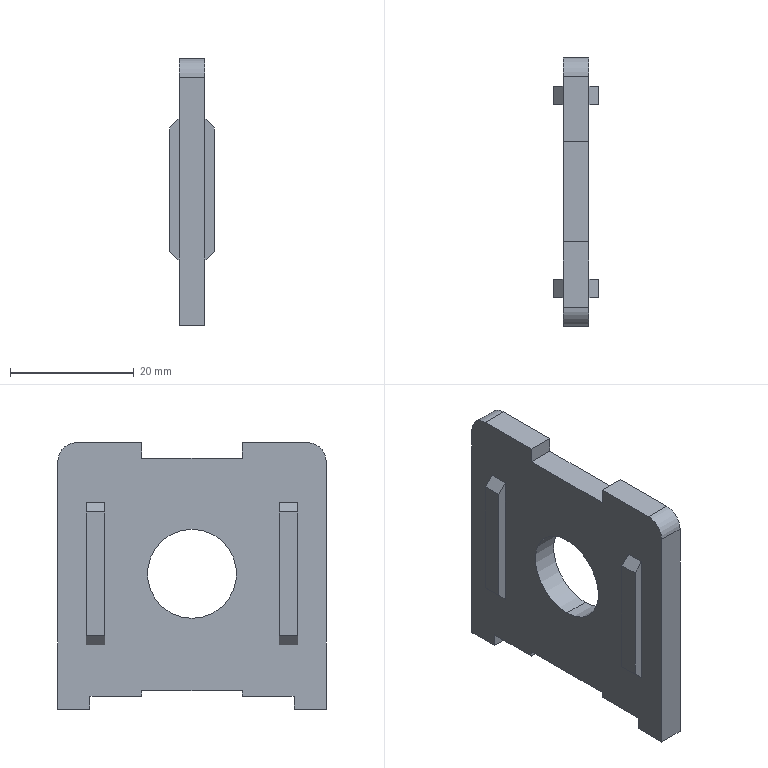Part | STEP file | _Y300T-A_SCREW | 1 solid | 42 faces | box 7.2 x 43.4 x 43.1 mm | volume 7021 mm3 | plane 38 | cylinder 4 | commonest cylinder face diameters 6 x2 14.4 x2
STEP:
#1=CARTESIAN_POINT('',(-2.1,0.,-7.2));
#2=VERTEX_POINT('',#1);
#3=CARTESIAN_POINT('',(-2.1,0.,7.2));
#4=VERTEX_POINT('',#3);
#5=CARTESIAN_POINT('',(-2.1,0.,0.));
#6=DIRECTION('',(-1.,0.,0.));
#7=DIRECTION('',(0.,0.,-1.));
#8=AXIS2_PLACEMENT_3D('',#5,#6,#7);
#9=CIRCLE('',#8,7.2);
#10=EDGE_CURVE('',#2,#4,#9,.T.);
#11=ORIENTED_EDGE('',*,*,#10,.T.);
#12=CARTESIAN_POINT('',(2.1,0.,7.2));
#13=VERTEX_POINT('',#12);
#14=CARTESIAN_POINT('',(2.1,0.,7.2));
#15=DIRECTION('',(1.,0.,0.));
#16=VECTOR('',#15,1000.);
#17=LINE('',#14,#16);
#18=EDGE_CURVE('',#4,#13,#17,.T.);
#19=ORIENTED_EDGE('',*,*,#18,.T.);
#20=CARTESIAN_POINT('',(2.1,0.,-7.2));
#21=VERTEX_POINT('',#20);
#22=CARTESIAN_POINT('',(2.1,0.,0.));
#23=DIRECTION('',(-1.,0.,0.));
#24=DIRECTION('',(0.,0.,-1.));
#25=AXIS2_PLACEMENT_3D('',#22,#23,#24);
#26=CIRCLE('',#25,7.2);
#27=EDGE_CURVE('',#21,#13,#26,.T.);
#28=ORIENTED_EDGE('',*,*,#27,.F.);
#29=CARTESIAN_POINT('',(2.1,0.,-7.2));
#30=DIRECTION('',(1.,0.,0.));
#31=VECTOR('',#30,1000.);
#32=LINE('',#29,#31);
#33=EDGE_CURVE('',#2,#21,#32,.T.);
#34=ORIENTED_EDGE('',*,*,#33,.F.);
#35=EDGE_LOOP('',(#11,#19,#28,#34));
#36=FACE_OUTER_BOUND('',#35,.T.);
#37=CARTESIAN_POINT('',(2.1,0.,0.));
#38=DIRECTION('',(1.,0.,0.));
#39=DIRECTION('',(0.,0.,-1.));
#40=AXIS2_PLACEMENT_3D('',#37,#38,#39);
#41=CYLINDRICAL_SURFACE('',#40,7.2);
#42=ADVANCED_FACE('',(#36),#41,.F.);
#43=CARTESIAN_POINT('',(-2.1,-14.1,-11.5));
#44=VERTEX_POINT('',#43);
#45=CARTESIAN_POINT('',(-2.1,-17.1,-11.5));
#46=VERTEX_POINT('',#45);
#47=CARTESIAN_POINT('',(-2.1,0.,-11.5));
#48=DIRECTION('',(0.,-1.,0.));
#49=VECTOR('',#48,1000.);
#50=LINE('',#47,#49);
#51=EDGE_CURVE('',#44,#46,#50,.T.);
#52=ORIENTED_EDGE('',*,*,#51,.F.);
#53=CARTESIAN_POINT('',(-2.1,-14.1,11.5));
#54=VERTEX_POINT('',#53);
#55=CARTESIAN_POINT('',(-2.1,-14.1,0.));
#56=DIRECTION('',(0.,0.,-1.));
#57=VECTOR('',#56,1000.);
#58=LINE('',#55,#57);
#59=EDGE_CURVE('',#54,#44,#58,.T.);
#60=ORIENTED_EDGE('',*,*,#59,.F.);
#61=CARTESIAN_POINT('',(-2.1,-17.1,11.5));
#62=VERTEX_POINT('',#61);
#63=CARTESIAN_POINT('',(-2.1,0.,11.5));
#64=DIRECTION('',(0.,1.,0.));
#65=VECTOR('',#64,1000.);
#66=LINE('',#63,#65);
#67=EDGE_CURVE('',#62,#54,#66,.T.);
#68=ORIENTED_EDGE('',*,*,#67,.F.);
#69=CARTESIAN_POINT('',(-2.1,-17.1,0.));
#70=DIRECTION('',(0.,0.,1.));
#71=VECTOR('',#70,1000.);
#72=LINE('',#69,#71);
#73=EDGE_CURVE('',#46,#62,#72,.T.);
#74=ORIENTED_EDGE('',*,*,#73,.F.);
#75=EDGE_LOOP('',(#52,#60,#68,#74));
#76=FACE_BOUND('',#75,.T.);
#77=CARTESIAN_POINT('',(-2.1,14.1,11.5));
#78=VERTEX_POINT('',#77);
#79=CARTESIAN_POINT('',(-2.1,17.1,11.5));
#80=VERTEX_POINT('',#79);
#81=CARTESIAN_POINT('',(-2.1,0.,11.5));
#82=DIRECTION('',(0.,1.,0.));
#83=VECTOR('',#82,1000.);
#84=LINE('',#81,#83);
#85=EDGE_CURVE('',#78,#80,#84,.T.);
#86=ORIENTED_EDGE('',*,*,#85,.F.);
#87=CARTESIAN_POINT('',(-2.1,14.1,-11.5));
#88=VERTEX_POINT('',#87);
#89=CARTESIAN_POINT('',(-2.1,14.1,0.));
#90=DIRECTION('',(0.,0.,1.));
#91=VECTOR('',#90,1000.);
#92=LINE('',#89,#91);
#93=EDGE_CURVE('',#88,#78,#92,.T.);
#94=ORIENTED_EDGE('',*,*,#93,.F.);
#95=CARTESIAN_POINT('',(-2.1,17.1,-11.5));
#96=VERTEX_POINT('',#95);
#97=CARTESIAN_POINT('',(-2.1,0.,-11.5));
#98=DIRECTION('',(0.,-1.,0.));
#99=VECTOR('',#98,1000.);
#100=LINE('',#97,#99);
#101=EDGE_CURVE('',#96,#88,#100,.T.);
#102=ORIENTED_EDGE('',*,*,#101,.F.);
#103=CARTESIAN_POINT('',(-2.1,17.1,0.));
#104=DIRECTION('',(0.,0.,-1.));
#105=VECTOR('',#104,1000.);
#106=LINE('',#103,#105);
#107=EDGE_CURVE('',#80,#96,#106,.T.);
#108=ORIENTED_EDGE('',*,*,#107,.F.);
#109=EDGE_LOOP('',(#86,#94,#102,#108));
#110=FACE_BOUND('',#109,.T.);
#111=ORIENTED_EDGE('',*,*,#10,.F.);
#112=CARTESIAN_POINT('',(-2.1,0.,0.));
#113=DIRECTION('',(-1.,0.,0.));
#114=DIRECTION('',(0.,0.,-1.));
#115=AXIS2_PLACEMENT_3D('',#112,#113,#114);
#116=CIRCLE('',#115,7.2);
#117=EDGE_CURVE('',#4,#2,#116,.T.);
#118=ORIENTED_EDGE('',*,*,#117,.F.);
#119=EDGE_LOOP('',(#111,#118));
#120=FACE_BOUND('',#119,.T.);
#121=CARTESIAN_POINT('',(-2.1,-16.5,-21.9));
#122=VERTEX_POINT('',#121);
#123=CARTESIAN_POINT('',(-2.1,-16.5,-19.8));
#124=VERTEX_POINT('',#123);
#125=CARTESIAN_POINT('',(-2.1,-16.5,0.));
#126=DIRECTION('',(0.,0.,1.));
#127=VECTOR('',#126,1000.);
#128=LINE('',#125,#127);
#129=EDGE_CURVE('',#122,#124,#128,.T.);
#130=ORIENTED_EDGE('',*,*,#129,.F.);
#131=CARTESIAN_POINT('',(-2.1,-21.7,-21.9));
#132=VERTEX_POINT('',#131);
#133=CARTESIAN_POINT('',(-2.1,0.,-21.9));
#134=DIRECTION('',(0.,1.,0.));
#135=VECTOR('',#134,1000.);
#136=LINE('',#133,#135);
#137=EDGE_CURVE('',#132,#122,#136,.T.);
#138=ORIENTED_EDGE('',*,*,#137,.F.);
#139=CARTESIAN_POINT('',(-2.1,-21.7,18.2));
#140=VERTEX_POINT('',#139);
#141=CARTESIAN_POINT('',(-2.1,-21.7,0.));
#142=DIRECTION('',(0.,0.,-1.));
#143=VECTOR('',#142,1000.);
#144=LINE('',#141,#143);
#145=EDGE_CURVE('',#140,#132,#144,.T.);
#146=ORIENTED_EDGE('',*,*,#145,.F.);
#147=CARTESIAN_POINT('',(-2.1,-18.7,21.2));
#148=VERTEX_POINT('',#147);
#149=CARTESIAN_POINT('',(-2.1,-18.7,18.2));
#150=DIRECTION('',(1.,0.,0.));
#151=DIRECTION('',(0.,0.,-1.));
#152=AXIS2_PLACEMENT_3D('',#149,#150,#151);
#153=CIRCLE('',#152,3.);
#154=EDGE_CURVE('',#148,#140,#153,.T.);
#155=ORIENTED_EDGE('',*,*,#154,.F.);
#156=CARTESIAN_POINT('',(-2.1,-8.1,21.2));
#157=VERTEX_POINT('',#156);
#158=CARTESIAN_POINT('',(-2.1,0.,21.2));
#159=DIRECTION('',(0.,-1.,0.));
#160=VECTOR('',#159,1000.);
#161=LINE('',#158,#160);
#162=EDGE_CURVE('',#157,#148,#161,.T.);
#163=ORIENTED_EDGE('',*,*,#162,.F.);
#164=CARTESIAN_POINT('',(-2.1,-8.1,18.7));
#165=VERTEX_POINT('',#164);
#166=CARTESIAN_POINT('',(-2.1,-8.1,0.));
#167=DIRECTION('',(0.,0.,1.));
#168=VECTOR('',#167,1000.);
#169=LINE('',#166,#168);
#170=EDGE_CURVE('',#165,#157,#169,.T.);
#171=ORIENTED_EDGE('',*,*,#170,.F.);
#172=CARTESIAN_POINT('',(-2.1,8.1,18.7));
#173=VERTEX_POINT('',#172);
#174=CARTESIAN_POINT('',(-2.1,0.,18.7));
#175=DIRECTION('',(0.,-1.,0.));
#176=VECTOR('',#175,1000.);
#177=LINE('',#174,#176);
#178=EDGE_CURVE('',#173,#165,#177,.T.);
#179=ORIENTED_EDGE('',*,*,#178,.F.);
#180=CARTESIAN_POINT('',(-2.1,8.1,21.2));
#181=VERTEX_POINT('',#180);
#182=CARTESIAN_POINT('',(-2.1,8.1,0.));
#183=DIRECTION('',(0.,0.,-1.));
#184=VECTOR('',#183,1000.);
#185=LINE('',#182,#184);
#186=EDGE_CURVE('',#181,#173,#185,.T.);
#187=ORIENTED_EDGE('',*,*,#186,.F.);
#188=CARTESIAN_POINT('',(-2.1,18.7,21.2));
#189=VERTEX_POINT('',#188);
#190=CARTESIAN_POINT('',(-2.1,0.,21.2));
#191=DIRECTION('',(0.,-1.,0.));
#192=VECTOR('',#191,1000.);
#193=LINE('',#190,#192);
#194=EDGE_CURVE('',#189,#181,#193,.T.);
#195=ORIENTED_EDGE('',*,*,#194,.F.);
#196=CARTESIAN_POINT('',(-2.1,21.7,18.2));
#197=VERTEX_POINT('',#196);
#198=CARTESIAN_POINT('',(-2.1,18.7,18.2));
#199=DIRECTION('',(1.,0.,0.));
#200=DIRECTION('',(0.,0.,-1.));
#201=AXIS2_PLACEMENT_3D('',#198,#199,#200);
#202=CIRCLE('',#201,3.);
#203=EDGE_CURVE('',#197,#189,#202,.T.);
#204=ORIENTED_EDGE('',*,*,#203,.F.);
#205=CARTESIAN_POINT('',(-2.1,21.7,-21.9));
#206=VERTEX_POINT('',#205);
#207=CARTESIAN_POINT('',(-2.1,21.7,0.));
#208=DIRECTION('',(0.,0.,1.));
#209=VECTOR('',#208,1000.);
#210=LINE('',#207,#209);
#211=EDGE_CURVE('',#206,#197,#210,.T.);
#212=ORIENTED_EDGE('',*,*,#211,.F.);
#213=CARTESIAN_POINT('',(-2.1,16.5,-21.9));
#214=VERTEX_POINT('',#213);
#215=CARTESIAN_POINT('',(-2.1,0.,-21.9));
#216=DIRECTION('',(0.,1.,0.));
#217=VECTOR('',#216,1000.);
#218=LINE('',#215,#217);
#219=EDGE_CURVE('',#214,#206,#218,.T.);
#220=ORIENTED_EDGE('',*,*,#219,.F.);
#221=CARTESIAN_POINT('',(-2.1,16.5,-19.8));
#222=VERTEX_POINT('',#221);
#223=CARTESIAN_POINT('',(-2.1,16.5,0.));
#224=DIRECTION('',(0.,0.,-1.));
#225=VECTOR('',#224,1000.);
#226=LINE('',#223,#225);
#227=EDGE_CURVE('',#222,#214,#226,.T.);
#228=ORIENTED_EDGE('',*,*,#227,.F.);
#229=CARTESIAN_POINT('',(-2.1,8.1,-19.8));
#230=VERTEX_POINT('',#229);
#231=CARTESIAN_POINT('',(-2.1,0.,-19.8));
#232=DIRECTION('',(0.,1.,0.));
#233=VECTOR('',#232,1000.);
#234=LINE('',#231,#233);
#235=EDGE_CURVE('',#230,#222,#234,.T.);
#236=ORIENTED_EDGE('',*,*,#235,.F.);
#237=CARTESIAN_POINT('',(-2.1,8.1,-18.9));
#238=VERTEX_POINT('',#237);
#239=CARTESIAN_POINT('',(-2.1,8.1,-18.9));
#240=DIRECTION('',(0.,0.,1.));
#241=VECTOR('',#240,1000.);
#242=LINE('',#239,#241);
#243=EDGE_CURVE('',#230,#238,#242,.T.);
#244=ORIENTED_EDGE('',*,*,#243,.T.);
#245=CARTESIAN_POINT('',(-2.1,-8.1,-18.9));
#246=VERTEX_POINT('',#245);
#247=CARTESIAN_POINT('',(-2.1,0.,-18.9));
#248=DIRECTION('',(0.,1.,0.));
#249=VECTOR('',#248,1000.);
#250=LINE('',#247,#249);
#251=EDGE_CURVE('',#246,#238,#250,.T.);
#252=ORIENTED_EDGE('',*,*,#251,.F.);
#253=CARTESIAN_POINT('',(-2.1,-8.1,-19.8));
#254=VERTEX_POINT('',#253);
#255=CARTESIAN_POINT('',(-2.1,-8.1,-21.9));
#256=DIRECTION('',(0.,0.,-1.));
#257=VECTOR('',#256,1000.);
#258=LINE('',#255,#257);
#259=EDGE_CURVE('',#246,#254,#258,.T.);
#260=ORIENTED_EDGE('',*,*,#259,.T.);
#261=CARTESIAN_POINT('',(-2.1,0.,-19.8));
#262=DIRECTION('',(0.,1.,0.));
#263=VECTOR('',#262,1000.);
#264=LINE('',#261,#263);
#265=EDGE_CURVE('',#124,#254,#264,.T.);
#266=ORIENTED_EDGE('',*,*,#265,.F.);
#267=EDGE_LOOP('',(#130,#138,#146,#155,#163,#171,#179,#187,#195,#204,#212,#220,#228,#236,#244,#252,#260,#266));
#268=FACE_OUTER_BOUND('',#267,.T.);
#269=CARTESIAN_POINT('',(-2.1,0.,0.));
#270=DIRECTION('',(1.,0.,0.));
#271=DIRECTION('',(0.,0.,-1.));
#272=AXIS2_PLACEMENT_3D('',#269,#270,#271);
#273=PLANE('',#272);
#274=ADVANCED_FACE('',(#76,#110,#120,#268),#273,.F.);
#275=CARTESIAN_POINT('',(-3.6,-17.1,-10.));
#276=VERTEX_POINT('',#275);
#277=CARTESIAN_POINT('',(-3.6,-17.1,10.));
#278=VERTEX_POINT('',#277);
#279=CARTESIAN_POINT('',(-3.6,-17.1,11.5));
#280=DIRECTION('',(0.,0.,1.));
#281=VECTOR('',#280,1000.);
#282=LINE('',#279,#281);
#283=EDGE_CURVE('',#276,#278,#282,.T.);
#284=ORIENTED_EDGE('',*,*,#283,.F.);
#285=CARTESIAN_POINT('',(-2.1,-17.1,-11.5));
#286=DIRECTION('',(-0.7071,0.,0.7071));
#287=VECTOR('',#286,1000.);
#288=LINE('',#285,#287);
#289=EDGE_CURVE('',#46,#276,#288,.T.);
#290=ORIENTED_EDGE('',*,*,#289,.F.);
#291=ORIENTED_EDGE('',*,*,#73,.T.);
#292=CARTESIAN_POINT('',(-3.6,-17.1,10.));
#293=DIRECTION('',(0.7071,0.,0.7071));
#294=VECTOR('',#293,1000.);
#295=LINE('',#292,#294);
#296=EDGE_CURVE('',#278,#62,#295,.T.);
#297=ORIENTED_EDGE('',*,*,#296,.F.);
#298=EDGE_LOOP('',(#284,#290,#291,#297));
#299=FACE_OUTER_BOUND('',#298,.T.);
#300=CARTESIAN_POINT('',(2.1,-17.1,11.5));
#301=DIRECTION('',(0.,1.,0.));
#302=DIRECTION('',(0.,0.,1.));
#303=AXIS2_PLACEMENT_3D('',#300,#301,#302);
#304=PLANE('',#303);
#305=ADVANCED_FACE('',(#299),#304,.F.);
#306=CARTESIAN_POINT('',(-3.6,-14.1,-10.));
#307=VERTEX_POINT('',#306);
#308=CARTESIAN_POINT('',(-2.1,-14.1,-11.5));
#309=DIRECTION('',(-0.7071,0.,0.7071));
#310=VECTOR('',#309,1000.);
#311=LINE('',#308,#310);
#312=EDGE_CURVE('',#44,#307,#311,.T.);
#313=ORIENTED_EDGE('',*,*,#312,.F.);
#314=ORIENTED_EDGE('',*,*,#51,.T.);
#315=ORIENTED_EDGE('',*,*,#289,.T.);
#316=CARTESIAN_POINT('',(-3.6,-14.1,-10.));
#317=DIRECTION('',(0.,-1.,0.));
#318=VECTOR('',#317,1000.);
#319=LINE('',#316,#318);
#320=EDGE_CURVE('',#307,#276,#319,.T.);
#321=ORIENTED_EDGE('',*,*,#320,.F.);
#322=EDGE_LOOP('',(#313,#314,#315,#321));
#323=FACE_OUTER_BOUND('',#322,.T.);
#324=CARTESIAN_POINT('',(-2.1,-14.1,-11.5));
#325=DIRECTION('',(0.7071,0.,0.7071));
#326=DIRECTION('',(0.7071,0.,-0.7071));
#327=AXIS2_PLACEMENT_3D('',#324,#325,#326);
#328=PLANE('',#327);
#329=ADVANCED_FACE('',(#323),#328,.F.);
#330=ORIENTED_EDGE('',*,*,#59,.T.);
#331=ORIENTED_EDGE('',*,*,#312,.T.);
#332=CARTESIAN_POINT('',(-3.6,-14.1,10.));
#333=VERTEX_POINT('',#332);
#334=CARTESIAN_POINT('',(-3.6,-14.1,0.));
#335=DIRECTION('',(0.,0.,1.));
#336=VECTOR('',#335,1000.);
#337=LINE('',#334,#336);
#338=EDGE_CURVE('',#307,#333,#337,.T.);
#339=ORIENTED_EDGE('',*,*,#338,.T.);
#340=CARTESIAN_POINT('',(-3.6,-14.1,10.));
#341=DIRECTION('',(0.7071,0.,0.7071));
#342=VECTOR('',#341,1000.);
#343=LINE('',#340,#342);
#344=EDGE_CURVE('',#333,#54,#343,.T.);
#345=ORIENTED_EDGE('',*,*,#344,.T.);
#346=EDGE_LOOP('',(#330,#331,#339,#345));
#347=FACE_OUTER_BOUND('',#346,.T.);
#348=CARTESIAN_POINT('',(0.,-14.1,0.));
#349=DIRECTION('',(0.,1.,0.));
#350=DIRECTION('',(0.,0.,1.));
#351=AXIS2_PLACEMENT_3D('',#348,#349,#350);
#352=PLANE('',#351);
#353=ADVANCED_FACE('',(#347),#352,.T.);
#354=ORIENTED_EDGE('',*,*,#344,.F.);
#355=CARTESIAN_POINT('',(-3.6,-14.1,10.));
#356=DIRECTION('',(0.,1.,0.));
#357=VECTOR('',#356,1000.);
#358=LINE('',#355,#357);
#359=EDGE_CURVE('',#278,#333,#358,.T.);
#360=ORIENTED_EDGE('',*,*,#359,.F.);
#361=ORIENTED_EDGE('',*,*,#296,.T.);
#362=ORIENTED_EDGE('',*,*,#67,.T.);
#363=EDGE_LOOP('',(#354,#360,#361,#362));
#364=FACE_OUTER_BOUND('',#363,.T.);
#365=CARTESIAN_POINT('',(-3.6,-14.1,10.));
#366=DIRECTION('',(0.7071,0.,-0.7071));
#367=DIRECTION('',(-0.7071,0.,-0.7071));
#368=AXIS2_PLACEMENT_3D('',#365,#366,#367);
#369=PLANE('',#368);
#370=ADVANCED_FACE('',(#364),#369,.F.);
#371=CARTESIAN_POINT('',(-3.6,17.1,10.));
#372=VERTEX_POINT('',#371);
#373=CARTESIAN_POINT('',(-3.6,17.1,-10.));
#374=VERTEX_POINT('',#373);
#375=CARTESIAN_POINT('',(-3.6,17.1,-21.9));
#376=DIRECTION('',(0.,0.,-1.));
#377=VECTOR('',#376,1000.);
#378=LINE('',#375,#377);
#379=EDGE_CURVE('',#372,#374,#378,.T.);
#380=ORIENTED_EDGE('',*,*,#379,.F.);
#381=CARTESIAN_POINT('',(-2.1,17.1,11.5));
#382=DIRECTION('',(-0.7071,0.,-0.7071));
#383=VECTOR('',#382,1000.);
#384=LINE('',#381,#383);
#385=EDGE_CURVE('',#80,#372,#384,.T.);
#386=ORIENTED_EDGE('',*,*,#385,.F.);
#387=ORIENTED_EDGE('',*,*,#107,.T.);
#388=CARTESIAN_POINT('',(-3.6,17.1,-10.));
#389=DIRECTION('',(0.7071,0.,-0.7071));
#390=VECTOR('',#389,1000.);
#391=LINE('',#388,#390);
#392=EDGE_CURVE('',#374,#96,#391,.T.);
#393=ORIENTED_EDGE('',*,*,#392,.F.);
#394=EDGE_LOOP('',(#380,#386,#387,#393));
#395=FACE_OUTER_BOUND('',#394,.T.);
#396=CARTESIAN_POINT('',(2.1,17.1,-21.9));
#397=DIRECTION('',(0.,-1.,0.));
#398=DIRECTION('',(0.,0.,-1.));
#399=AXIS2_PLACEMENT_3D('',#396,#397,#398);
#400=PLANE('',#399);
#401=ADVANCED_FACE('',(#395),#400,.F.);
#402=ORIENTED_EDGE('',*,*,#385,.T.);
#403=CARTESIAN_POINT('',(-3.6,14.1,10.));
#404=VERTEX_POINT('',#403);
#405=CARTESIAN_POINT('',(-3.6,14.1,10.));
#406=DIRECTION('',(0.,-1.,0.));
#407=VECTOR('',#406,1000.);
#408=LINE('',#405,#407);
#409=EDGE_CURVE('',#372,#404,#408,.T.);
#410=ORIENTED_EDGE('',*,*,#409,.T.);
#411=CARTESIAN_POINT('',(-3.6,14.1,10.));
#412=DIRECTION('',(0.7071,0.,0.7071));
#413=VECTOR('',#412,1000.);
#414=LINE('',#411,#413);
#415=EDGE_CURVE('',#404,#78,#414,.T.);
#416=ORIENTED_EDGE('',*,*,#415,.T.);
#417=ORIENTED_EDGE('',*,*,#85,.T.);
#418=EDGE_LOOP('',(#402,#410,#416,#417));
#419=FACE_OUTER_BOUND('',#418,.T.);
#420=CARTESIAN_POINT('',(-3.6,14.1,10.));
#421=DIRECTION('',(-0.7071,0.,0.7071));
#422=DIRECTION('',(0.7071,0.,0.7071));
#423=AXIS2_PLACEMENT_3D('',#420,#421,#422);
#424=PLANE('',#423);
#425=ADVANCED_FACE('',(#419),#424,.T.);
#426=ORIENTED_EDGE('',*,*,#415,.F.);
#427=CARTESIAN_POINT('',(-3.6,14.1,-10.));
#428=VERTEX_POINT('',#427);
#429=CARTESIAN_POINT('',(-3.6,14.1,0.));
#430=DIRECTION('',(0.,0.,1.));
#431=VECTOR('',#430,1000.);
#432=LINE('',#429,#431);
#433=EDGE_CURVE('',#428,#404,#432,.T.);
#434=ORIENTED_EDGE('',*,*,#433,.F.);
#435=CARTESIAN_POINT('',(-2.1,14.1,-11.5));
#436=DIRECTION('',(-0.7071,0.,0.7071));
#437=VECTOR('',#436,1000.);
#438=LINE('',#435,#437);
#439=EDGE_CURVE('',#88,#428,#438,.T.);
#440=ORIENTED_EDGE('',*,*,#439,.F.);
#441=ORIENTED_EDGE('',*,*,#93,.T.);
#442=EDGE_LOOP('',(#426,#434,#440,#441));
#443=FACE_OUTER_BOUND('',#442,.T.);
#444=CARTESIAN_POINT('',(0.,14.1,0.));
#445=DIRECTION('',(0.,1.,0.));
#446=DIRECTION('',(0.,0.,1.));
#447=AXIS2_PLACEMENT_3D('',#444,#445,#446);
#448=PLANE('',#447);
#449=ADVANCED_FACE('',(#443),#448,.F.);
#450=ORIENTED_EDGE('',*,*,#392,.T.);
#451=ORIENTED_EDGE('',*,*,#101,.T.);
#452=ORIENTED_EDGE('',*,*,#439,.T.);
#453=CARTESIAN_POINT('',(-3.6,14.1,-10.));
#454=DIRECTION('',(0.,1.,0.));
#455=VECTOR('',#454,1000.);
#456=LINE('',#453,#455);
#457=EDGE_CURVE('',#428,#374,#456,.T.);
#458=ORIENTED_EDGE('',*,*,#457,.T.);
#459=EDGE_LOOP('',(#450,#451,#452,#458));
#460=FACE_OUTER_BOUND('',#459,.T.);
#461=CARTESIAN_POINT('',(-2.1,14.1,-11.5));
#462=DIRECTION('',(-0.7071,0.,-0.7071));
#463=DIRECTION('',(-0.7071,0.,0.7071));
#464=AXIS2_PLACEMENT_3D('',#461,#462,#463);
#465=PLANE('',#464);
#466=ADVANCED_FACE('',(#460),#465,.T.);
#467=ORIENTED_EDGE('',*,*,#18,.F.);
#468=ORIENTED_EDGE('',*,*,#117,.T.);
#469=ORIENTED_EDGE('',*,*,#33,.T.);
#470=CARTESIAN_POINT('',(2.1,0.,0.));
#471=DIRECTION('',(-1.,0.,0.));
#472=DIRECTION('',(0.,0.,-1.));
#473=AXIS2_PLACEMENT_3D('',#470,#471,#472);
#474=CIRCLE('',#473,7.2);
#475=EDGE_CURVE('',#13,#21,#474,.T.);
#476=ORIENTED_EDGE('',*,*,#475,.F.);
#477=EDGE_LOOP('',(#467,#468,#469,#476));
#478=FACE_OUTER_BOUND('',#477,.T.);
#479=CARTESIAN_POINT('',(2.1,0.,0.));
#480=DIRECTION('',(1.,0.,0.));
#481=DIRECTION('',(0.,0.,-1.));
#482=AXIS2_PLACEMENT_3D('',#479,#480,#481);
#483=CYLINDRICAL_SURFACE('',#482,7.2);
#484=ADVANCED_FACE('',(#478),#483,.F.);
#485=CARTESIAN_POINT('',(2.1,-16.5,-19.8));
#486=VERTEX_POINT('',#485);
#487=CARTESIAN_POINT('',(2.1,-8.1,-19.8));
#488=VERTEX_POINT('',#487);
#489=CARTESIAN_POINT('',(2.1,-14.5,-19.8));
#490=DIRECTION('',(0.,1.,0.));
#491=VECTOR('',#490,1000.);
#492=LINE('',#489,#491);
#493=EDGE_CURVE('',#486,#488,#492,.T.);
#494=ORIENTED_EDGE('',*,*,#493,.F.);
#495=CARTESIAN_POINT('',(2.1,-16.5,-19.8));
#496=DIRECTION('',(1.,0.,0.));
#497=VECTOR('',#496,1000.);
#498=LINE('',#495,#497);
#499=EDGE_CURVE('',#124,#486,#498,.T.);
#500=ORIENTED_EDGE('',*,*,#499,.F.);
#501=ORIENTED_EDGE('',*,*,#265,.T.);
#502=CARTESIAN_POINT('',(2.1,-8.1,-19.8));
#503=DIRECTION('',(-1.,0.,0.));
#504=VECTOR('',#503,1000.);
#505=LINE('',#502,#504);
#506=EDGE_CURVE('',#488,#254,#505,.T.);
#507=ORIENTED_EDGE('',*,*,#506,.F.);
#508=EDGE_LOOP('',(#494,#500,#501,#507));
#509=FACE_OUTER_BOUND('',#508,.T.);
#510=CARTESIAN_POINT('',(2.1,-14.5,-19.8));
#511=DIRECTION('',(0.,0.,1.));
#512=DIRECTION('',(1.,0.,0.));
#513=AXIS2_PLACEMENT_3D('',#510,#511,#512);
#514=PLANE('',#513);
#515=ADVANCED_FACE('',(#509),#514,.F.);
#516=ORIENTED_EDGE('',*,*,#129,.T.);
#517=ORIENTED_EDGE('',*,*,#499,.T.);
#518=CARTESIAN_POINT('',(2.1,-16.5,-21.9));
#519=VERTEX_POINT('',#518);
#520=CARTESIAN_POINT('',(2.1,-16.5,-19.8));
#521=DIRECTION('',(0.,0.,-1.));
#522=VECTOR('',#521,1000.);
#523=LINE('',#520,#522);
#524=EDGE_CURVE('',#486,#519,#523,.T.);
#525=ORIENTED_EDGE('',*,*,#524,.T.);
#526=CARTESIAN_POINT('',(2.1,-16.5,-21.9));
#527=DIRECTION('',(-1.,0.,0.));
#528=VECTOR('',#527,1000.);
#529=LINE('',#526,#528);
#530=EDGE_CURVE('',#519,#122,#529,.T.);
#531=ORIENTED_EDGE('',*,*,#530,.T.);
#532=EDGE_LOOP('',(#516,#517,#525,#531));
#533=FACE_OUTER_BOUND('',#532,.T.);
#534=CARTESIAN_POINT('',(2.1,-16.5,-19.8));
#535=DIRECTION('',(0.,1.,0.));
#536=DIRECTION('',(0.,0.,1.));
#537=AXIS2_PLACEMENT_3D('',#534,#535,#536);
#538=PLANE('',#537);
#539=ADVANCED_FACE('',(#533),#538,.T.);
#540=CARTESIAN_POINT('',(2.1,-21.7,-21.9));
#541=VERTEX_POINT('',#540);
#542=CARTESIAN_POINT('',(2.1,-21.7,-21.9));
#543=DIRECTION('',(1.,0.,0.));
#544=VECTOR('',#543,1000.);
#545=LINE('',#542,#544);
#546=EDGE_CURVE('',#132,#541,#545,.T.);
#547=ORIENTED_EDGE('',*,*,#546,.F.);
#548=ORIENTED_EDGE('',*,*,#137,.T.);
#549=ORIENTED_EDGE('',*,*,#530,.F.);
#550=CARTESIAN_POINT('',(2.1,-17.1,-21.9));
#551=DIRECTION('',(0.,1.,0.));
#552=VECTOR('',#551,1000.);
#553=LINE('',#550,#552);
#554=EDGE_CURVE('',#541,#519,#553,.T.);
#555=ORIENTED_EDGE('',*,*,#554,.F.);
#556=EDGE_LOOP('',(#547,#548,#549,#555));
#557=FACE_OUTER_BOUND('',#556,.T.);
#558=CARTESIAN_POINT('',(2.1,-17.1,-21.9));
#559=DIRECTION('',(0.,0.,1.));
#560=DIRECTION('',(1.,0.,0.));
#561=AXIS2_PLACEMENT_3D('',#558,#559,#560);
#562=PLANE('',#561);
#563=ADVANCED_FACE('',(#557),#562,.F.);
#564=CARTESIAN_POINT('',(2.1,-21.7,18.2));
#565=VERTEX_POINT('',#564);
#566=CARTESIAN_POINT('',(2.1,-21.7,18.2));
#567=DIRECTION('',(0.,0.,-1.));
#568=VECTOR('',#567,1000.);
#569=LINE('',#566,#568);
#570=EDGE_CURVE('',#565,#541,#569,.T.);
#571=ORIENTED_EDGE('',*,*,#570,.F.);
#572=CARTESIAN_POINT('',(2.1,-21.7,18.2));
#573=DIRECTION('',(1.,0.,0.));
#574=VECTOR('',#573,1000.);
#575=LINE('',#572,#574);
#576=EDGE_CURVE('',#140,#565,#575,.T.);
#577=ORIENTED_EDGE('',*,*,#576,.F.);
#578=ORIENTED_EDGE('',*,*,#145,.T.);
#579=ORIENTED_EDGE('',*,*,#546,.T.);
#580=EDGE_LOOP('',(#571,#577,#578,#579));
#581=FACE_OUTER_BOUND('',#580,.T.);
#582=CARTESIAN_POINT('',(2.1,-21.7,18.2));
#583=DIRECTION('',(0.,1.,0.));
#584=DIRECTION('',(0.,0.,1.));
#585=AXIS2_PLACEMENT_3D('',#582,#583,#584);
#586=PLANE('',#585);
#587=ADVANCED_FACE('',(#581),#586,.F.);
#588=ORIENTED_EDGE('',*,*,#154,.T.);
#589=ORIENTED_EDGE('',*,*,#576,.T.);
#590=CARTESIAN_POINT('',(2.1,-18.7,21.2));
#591=VERTEX_POINT('',#590);
#592=CARTESIAN_POINT('',(2.1,-18.7,18.2));
#593=DIRECTION('',(-1.,0.,0.));
#594=DIRECTION('',(0.,0.,-1.));
#595=AXIS2_PLACEMENT_3D('',#592,#593,#594);
#596=CIRCLE('',#595,3.);
#597=EDGE_CURVE('',#565,#591,#596,.T.);
#598=ORIENTED_EDGE('',*,*,#597,.T.);
#599=CARTESIAN_POINT('',(2.1,-18.7,21.2));
#600=DIRECTION('',(-1.,0.,0.));
#601=VECTOR('',#600,1000.);
#602=LINE('',#599,#601);
#603=EDGE_CURVE('',#591,#148,#602,.T.);
#604=ORIENTED_EDGE('',*,*,#603,.T.);
#605=EDGE_LOOP('',(#588,#589,#598,#604));
#606=FACE_OUTER_BOUND('',#605,.T.);
#607=CARTESIAN_POINT('',(2.1,-18.7,18.2));
#608=DIRECTION('',(1.,0.,0.));
#609=DIRECTION('',(0.,0.,-1.));
#610=AXIS2_PLACEMENT_3D('',#607,#608,#609);
#611=CYLINDRICAL_SURFACE('',#610,3.);
#612=ADVANCED_FACE('',(#606),#611,.T.);
#613=CARTESIAN_POINT('',(2.1,-8.1,21.2));
#614=VERTEX_POINT('',#613);
#615=CARTESIAN_POINT('',(2.1,-8.1,21.2));
#616=DIRECTION('',(0.,-1.,0.));
#617=VECTOR('',#616,1000.);
#618=LINE('',#615,#617);
#619=EDGE_CURVE('',#614,#591,#618,.T.);
#620=ORIENTED_EDGE('',*,*,#619,.F.);
#621=CARTESIAN_POINT('',(2.1,-8.1,21.2));
#622=DIRECTION('',(1.,0.,0.));
#623=VECTOR('',#622,1000.);
#624=LINE('',#621,#623);
#625=EDGE_CURVE('',#157,#614,#624,.T.);
#626=ORIENTED_EDGE('',*,*,#625,.F.);
#627=ORIENTED_EDGE('',*,*,#162,.T.);
#628=ORIENTED_EDGE('',*,*,#603,.F.);
#629=EDGE_LOOP('',(#620,#626,#627,#628));
#630=FACE_OUTER_BOUND('',#629,.T.);
#631=CARTESIAN_POINT('',(2.1,-8.1,21.2));
#632=DIRECTION('',(0.,0.,-1.));
#633=DIRECTION('',(-1.,0.,0.));
#634=AXIS2_PLACEMENT_3D('',#631,#632,#633);
#635=PLANE('',#634);
#636=ADVANCED_FACE('',(#630),#635,.F.);
#637=CARTESIAN_POINT('',(2.1,-8.1,18.7));
#638=VERTEX_POINT('',#637);
#639=CARTESIAN_POINT('',(2.1,-8.1,18.7));
#640=DIRECTION('',(0.,0.,1.));
#641=VECTOR('',#640,1000.);
#642=LINE('',#639,#641);
#643=EDGE_CURVE('',#638,#614,#642,.T.);
#644=ORIENTED_EDGE('',*,*,#643,.F.);
#645=CARTESIAN_POINT('',(2.1,-8.1,18.7));
#646=DIRECTION('',(1.,0.,0.));
#647=VECTOR('',#646,1000.);
#648=LINE('',#645,#647);
#649=EDGE_CURVE('',#165,#638,#648,.T.);
#650=ORIENTED_EDGE('',*,*,#649,.F.);
#651=ORIENTED_EDGE('',*,*,#170,.T.);
#652=ORIENTED_EDGE('',*,*,#625,.T.);
#653=EDGE_LOOP('',(#644,#650,#651,#652));
#654=FACE_OUTER_BOUND('',#653,.T.);
#655=CARTESIAN_POINT('',(2.1,-8.1,18.7));
#656=DIRECTION('',(0.,-1.,0.));
#657=DIRECTION('',(0.,0.,-1.));
#658=AXIS2_PLACEMENT_3D('',#655,#656,#657);
#659=PLANE('',#658);
#660=ADVANCED_FACE('',(#654),#659,.F.);
#661=CARTESIAN_POINT('',(2.1,8.1,18.7));
#662=VERTEX_POINT('',#661);
#663=CARTESIAN_POINT('',(2.1,8.1,18.7));
#664=DIRECTION('',(0.,-1.,0.));
#665=VECTOR('',#664,1000.);
#666=LINE('',#663,#665);
#667=EDGE_CURVE('',#662,#638,#666,.T.);
#668=ORIENTED_EDGE('',*,*,#667,.F.);
#669=CARTESIAN_POINT('',(2.1,8.1,18.7));
#670=DIRECTION('',(1.,0.,0.));
#671=VECTOR('',#670,1000.);
#672=LINE('',#669,#671);
#673=EDGE_CURVE('',#173,#662,#672,.T.);
#674=ORIENTED_EDGE('',*,*,#673,.F.);
#675=ORIENTED_EDGE('',*,*,#178,.T.);
#676=ORIENTED_EDGE('',*,*,#649,.T.);
#677=EDGE_LOOP('',(#668,#674,#675,#676));
#678=FACE_OUTER_BOUND('',#677,.T.);
#679=CARTESIAN_POINT('',(2.1,8.1,18.7));
#680=DIRECTION('',(0.,0.,-1.));
#681=DIRECTION('',(-1.,0.,0.));
#682=AXIS2_PLACEMENT_3D('',#679,#680,#681);
#683=PLANE('',#682);
#684=ADVANCED_FACE('',(#678),#683,.F.);
#685=CARTESIAN_POINT('',(2.1,8.1,21.2));
#686=VERTEX_POINT('',#685);
#687=CARTESIAN_POINT('',(2.1,8.1,21.2));
#688=DIRECTION('',(0.,0.,-1.));
#689=VECTOR('',#688,1000.);
#690=LINE('',#687,#689);
#691=EDGE_CURVE('',#686,#662,#690,.T.);
#692=ORIENTED_EDGE('',*,*,#691,.F.);
#693=CARTESIAN_POINT('',(2.1,8.1,21.2));
#694=DIRECTION('',(1.,0.,0.));
#695=VECTOR('',#694,1000.);
#696=LINE('',#693,#695);
#697=EDGE_CURVE('',#181,#686,#696,.T.);
#698=ORIENTED_EDGE('',*,*,#697,.F.);
#699=ORIENTED_EDGE('',*,*,#186,.T.);
#700=ORIENTED_EDGE('',*,*,#673,.T.);
#701=EDGE_LOOP('',(#692,#698,#699,#700));
#702=FACE_OUTER_BOUND('',#701,.T.);
#703=CARTESIAN_POINT('',(2.1,8.1,21.2));
#704=DIRECTION('',(0.,1.,0.));
#705=DIRECTION('',(0.,0.,1.));
#706=AXIS2_PLACEMENT_3D('',#703,#704,#705);
#707=PLANE('',#706);
#708=ADVANCED_FACE('',(#702),#707,.F.);
#709=CARTESIAN_POINT('',(2.1,18.7,21.2));
#710=VERTEX_POINT('',#709);
#711=CARTESIAN_POINT('',(2.1,13.569,21.2));
#712=DIRECTION('',(0.,-1.,0.));
#713=VECTOR('',#712,1000.);
#714=LINE('',#711,#713);
#715=EDGE_CURVE('',#710,#686,#714,.T.);
#716=ORIENTED_EDGE('',*,*,#715,.F.);
#717=CARTESIAN_POINT('',(2.1,18.7,21.2));
#718=DIRECTION('',(1.,0.,0.));
#719=VECTOR('',#718,1000.);
#720=LINE('',#717,#719);
#721=EDGE_CURVE('',#189,#710,#720,.T.);
#722=ORIENTED_EDGE('',*,*,#721,.F.);
#723=ORIENTED_EDGE('',*,*,#194,.T.);
#724=ORIENTED_EDGE('',*,*,#697,.T.);
#725=EDGE_LOOP('',(#716,#722,#723,#724));
#726=FACE_OUTER_BOUND('',#725,.T.);
#727=CARTESIAN_POINT('',(2.1,13.569,21.2));
#728=DIRECTION('',(0.,0.,-1.));
#729=DIRECTION('',(-1.,0.,0.));
#730=AXIS2_PLACEMENT_3D('',#727,#728,#729);
#731=PLANE('',#730);
#732=ADVANCED_FACE('',(#726),#731,.F.);
#733=ORIENTED_EDGE('',*,*,#203,.T.);
#734=ORIENTED_EDGE('',*,*,#721,.T.);
#735=CARTESIAN_POINT('',(2.1,21.7,18.2));
#736=VERTEX_POINT('',#735);
#737=CARTESIAN_POINT('',(2.1,18.7,18.2));
#738=DIRECTION('',(-1.,0.,0.));
#739=DIRECTION('',(0.,0.,-1.));
#740=AXIS2_PLACEMENT_3D('',#737,#738,#739);
#741=CIRCLE('',#740,3.);
#742=EDGE_CURVE('',#710,#736,#741,.T.);
#743=ORIENTED_EDGE('',*,*,#742,.T.);
#744=CARTESIAN_POINT('',(2.1,21.7,18.2));
#745=DIRECTION('',(-1.,0.,0.));
#746=VECTOR('',#745,1000.);
#747=LINE('',#744,#746);
#748=EDGE_CURVE('',#736,#197,#747,.T.);
#749=ORIENTED_EDGE('',*,*,#748,.T.);
#750=EDGE_LOOP('',(#733,#734,#743,#749));
#751=FACE_OUTER_BOUND('',#750,.T.);
#752=CARTESIAN_POINT('',(2.1,18.7,18.2));
#753=DIRECTION('',(1.,0.,0.));
#754=DIRECTION('',(0.,0.,-1.));
#755=AXIS2_PLACEMENT_3D('',#752,#753,#754);
#756=CYLINDRICAL_SURFACE('',#755,3.);
#757=ADVANCED_FACE('',(#751),#756,.T.);
#758=CARTESIAN_POINT('',(2.1,21.7,-21.9));
#759=VERTEX_POINT('',#758);
#760=CARTESIAN_POINT('',(2.1,21.7,-21.9));
#761=DIRECTION('',(0.,0.,1.));
#762=VECTOR('',#761,1000.);
#763=LINE('',#760,#762);
#764=EDGE_CURVE('',#759,#736,#763,.T.);
#765=ORIENTED_EDGE('',*,*,#764,.F.);
#766=CARTESIAN_POINT('',(2.1,21.7,-21.9));
#767=DIRECTION('',(1.,0.,0.));
#768=VECTOR('',#767,1000.);
#769=LINE('',#766,#768);
#770=EDGE_CURVE('',#206,#759,#769,.T.);
#771=ORIENTED_EDGE('',*,*,#770,.F.);
#772=ORIENTED_EDGE('',*,*,#211,.T.);
#773=ORIENTED_EDGE('',*,*,#748,.F.);
#774=EDGE_LOOP('',(#765,#771,#772,#773));
#775=FACE_OUTER_BOUND('',#774,.T.);
#776=CARTESIAN_POINT('',(2.1,21.7,-21.9));
#777=DIRECTION('',(0.,-1.,0.));
#778=DIRECTION('',(0.,0.,-1.));
#779=AXIS2_PLACEMENT_3D('',#776,#777,#778);
#780=PLANE('',#779);
#781=ADVANCED_FACE('',(#775),#780,.F.);
#782=ORIENTED_EDGE('',*,*,#770,.T.);
#783=CARTESIAN_POINT('',(2.1,16.5,-21.9));
#784=VERTEX_POINT('',#783);
#785=CARTESIAN_POINT('',(2.1,14.5,-21.9));
#786=DIRECTION('',(0.,1.,0.));
#787=VECTOR('',#786,1000.);
#788=LINE('',#785,#787);
#789=EDGE_CURVE('',#784,#759,#788,.T.);
#790=ORIENTED_EDGE('',*,*,#789,.F.);
#791=CARTESIAN_POINT('',(2.1,16.5,-21.9));
#792=DIRECTION('',(1.,0.,0.));
#793=VECTOR('',#792,1000.);
#794=LINE('',#791,#793);
#795=EDGE_CURVE('',#214,#784,#794,.T.);
#796=ORIENTED_EDGE('',*,*,#795,.F.);
#797=ORIENTED_EDGE('',*,*,#219,.T.);
#798=EDGE_LOOP('',(#782,#790,#796,#797));
#799=FACE_OUTER_BOUND('',#798,.T.);
#800=CARTESIAN_POINT('',(2.1,14.5,-21.9));
#801=DIRECTION('',(0.,0.,1.));
#802=DIRECTION('',(1.,0.,0.));
#803=AXIS2_PLACEMENT_3D('',#800,#801,#802);
#804=PLANE('',#803);
#805=ADVANCED_FACE('',(#799),#804,.F.);
#806=ORIENTED_EDGE('',*,*,#227,.T.);
#807=ORIENTED_EDGE('',*,*,#795,.T.);
#808=CARTESIAN_POINT('',(2.1,16.5,-19.8));
#809=VERTEX_POINT('',#808);
#810=CARTESIAN_POINT('',(2.1,16.5,-21.9));
#811=DIRECTION('',(0.,0.,1.));
#812=VECTOR('',#811,1000.);
#813=LINE('',#810,#812);
#814=EDGE_CURVE('',#784,#809,#813,.T.);
#815=ORIENTED_EDGE('',*,*,#814,.T.);
#816=CARTESIAN_POINT('',(2.1,16.5,-19.8));
#817=DIRECTION('',(-1.,0.,0.));
#818=VECTOR('',#817,1000.);
#819=LINE('',#816,#818);
#820=EDGE_CURVE('',#809,#222,#819,.T.);
#821=ORIENTED_EDGE('',*,*,#820,.T.);
#822=EDGE_LOOP('',(#806,#807,#815,#821));
#823=FACE_OUTER_BOUND('',#822,.T.);
#824=CARTESIAN_POINT('',(2.1,16.5,-21.9));
#825=DIRECTION('',(0.,-1.,0.));
#826=DIRECTION('',(0.,0.,-1.));
#827=AXIS2_PLACEMENT_3D('',#824,#825,#826);
#828=PLANE('',#827);
#829=ADVANCED_FACE('',(#823),#828,.T.);
#830=CARTESIAN_POINT('',(2.1,8.1,-19.8));
#831=VERTEX_POINT('',#830);
#832=CARTESIAN_POINT('',(2.1,12.,-19.8));
#833=DIRECTION('',(0.,1.,0.));
#834=VECTOR('',#833,1000.);
#835=LINE('',#832,#834);
#836=EDGE_CURVE('',#831,#809,#835,.T.);
#837=ORIENTED_EDGE('',*,*,#836,.F.);
#838=CARTESIAN_POINT('',(2.1,8.1,-19.8));
#839=DIRECTION('',(1.,0.,0.));
#840=VECTOR('',#839,1000.);
#841=LINE('',#838,#840);
#842=EDGE_CURVE('',#230,#831,#841,.T.);
#843=ORIENTED_EDGE('',*,*,#842,.F.);
#844=ORIENTED_EDGE('',*,*,#235,.T.);
#845=ORIENTED_EDGE('',*,*,#820,.F.);
#846=EDGE_LOOP('',(#837,#843,#844,#845));
#847=FACE_OUTER_BOUND('',#846,.T.);
#848=CARTESIAN_POINT('',(2.1,12.,-19.8));
#849=DIRECTION('',(0.,0.,1.));
#850=DIRECTION('',(1.,0.,0.));
#851=AXIS2_PLACEMENT_3D('',#848,#849,#850);
#852=PLANE('',#851);
#853=ADVANCED_FACE('',(#847),#852,.F.);
#854=CARTESIAN_POINT('',(2.1,-8.1,-18.9));
#855=VERTEX_POINT('',#854);
#856=CARTESIAN_POINT('',(2.1,8.1,-18.9));
#857=VERTEX_POINT('',#856);
#858=CARTESIAN_POINT('',(2.1,-8.1,-18.9));
#859=DIRECTION('',(0.,1.,0.));
#860=VECTOR('',#859,1000.);
#861=LINE('',#858,#860);
#862=EDGE_CURVE('',#855,#857,#861,.T.);
#863=ORIENTED_EDGE('',*,*,#862,.F.);
#864=CARTESIAN_POINT('',(2.1,-8.1,-18.9));
#865=DIRECTION('',(1.,0.,0.));
#866=VECTOR('',#865,1000.);
#867=LINE('',#864,#866);
#868=EDGE_CURVE('',#246,#855,#867,.T.);
#869=ORIENTED_EDGE('',*,*,#868,.F.);
#870=ORIENTED_EDGE('',*,*,#251,.T.);
#871=CARTESIAN_POINT('',(2.1,8.1,-18.9));
#872=DIRECTION('',(-1.,0.,0.));
#873=VECTOR('',#872,1000.);
#874=LINE('',#871,#873);
#875=EDGE_CURVE('',#857,#238,#874,.T.);
#876=ORIENTED_EDGE('',*,*,#875,.F.);
#877=EDGE_LOOP('',(#863,#869,#870,#876));
#878=FACE_OUTER_BOUND('',#877,.T.);
#879=CARTESIAN_POINT('',(2.1,-8.1,-18.9));
#880=DIRECTION('',(0.,0.,1.));
#881=DIRECTION('',(1.,0.,0.));
#882=AXIS2_PLACEMENT_3D('',#879,#880,#881);
#883=PLANE('',#882);
#884=ADVANCED_FACE('',(#878),#883,.F.);
#885=ORIENTED_EDGE('',*,*,#338,.F.);
#886=ORIENTED_EDGE('',*,*,#320,.T.);
#887=ORIENTED_EDGE('',*,*,#283,.T.);
#888=ORIENTED_EDGE('',*,*,#359,.T.);
#889=EDGE_LOOP('',(#885,#886,#887,#888));
#890=FACE_OUTER_BOUND('',#889,.T.);
#891=CARTESIAN_POINT('',(-3.6,-14.1,-10.));
#892=DIRECTION('',(1.,0.,0.));
#893=DIRECTION('',(0.,0.,-1.));
#894=AXIS2_PLACEMENT_3D('',#891,#892,#893);
#895=PLANE('',#894);
#896=ADVANCED_FACE('',(#890),#895,.F.);
#897=ORIENTED_EDGE('',*,*,#379,.T.);
#898=ORIENTED_EDGE('',*,*,#457,.F.);
#899=ORIENTED_EDGE('',*,*,#433,.T.);
#900=ORIENTED_EDGE('',*,*,#409,.F.);
#901=EDGE_LOOP('',(#897,#898,#899,#900));
#902=FACE_OUTER_BOUND('',#901,.T.);
#903=CARTESIAN_POINT('',(-3.6,14.1,-10.));
#904=DIRECTION('',(-1.,0.,0.));
#905=DIRECTION('',(0.,0.,1.));
#906=AXIS2_PLACEMENT_3D('',#903,#904,#905);
#907=PLANE('',#906);
#908=ADVANCED_FACE('',(#902),#907,.T.);
#909=CARTESIAN_POINT('',(2.1,-17.1,-11.5));
#910=VERTEX_POINT('',#909);
#911=CARTESIAN_POINT('',(2.1,-17.1,11.5));
#912=VERTEX_POINT('',#911);
#913=CARTESIAN_POINT('',(2.1,-17.1,0.));
#914=DIRECTION('',(0.,0.,1.));
#915=VECTOR('',#914,1000.);
#916=LINE('',#913,#915);
#917=EDGE_CURVE('',#910,#912,#916,.T.);
#918=ORIENTED_EDGE('',*,*,#917,.T.);
#919=CARTESIAN_POINT('',(2.1,-14.1,11.5));
#920=VERTEX_POINT('',#919);
#921=CARTESIAN_POINT('',(2.1,0.,11.5));
#922=DIRECTION('',(0.,1.,0.));
#923=VECTOR('',#922,1000.);
#924=LINE('',#921,#923);
#925=EDGE_CURVE('',#912,#920,#924,.T.);
#926=ORIENTED_EDGE('',*,*,#925,.T.);
#927=CARTESIAN_POINT('',(2.1,-14.1,-11.5));
#928=VERTEX_POINT('',#927);
#929=CARTESIAN_POINT('',(2.1,-14.1,0.));
#930=DIRECTION('',(0.,0.,-1.));
#931=VECTOR('',#930,1000.);
#932=LINE('',#929,#931);
#933=EDGE_CURVE('',#920,#928,#932,.T.);
#934=ORIENTED_EDGE('',*,*,#933,.T.);
#935=CARTESIAN_POINT('',(2.1,0.,-11.5));
#936=DIRECTION('',(0.,-1.,0.));
#937=VECTOR('',#936,1000.);
#938=LINE('',#935,#937);
#939=EDGE_CURVE('',#928,#910,#938,.T.);
#940=ORIENTED_EDGE('',*,*,#939,.T.);
#941=EDGE_LOOP('',(#918,#926,#934,#940));
#942=FACE_BOUND('',#941,.T.);
#943=CARTESIAN_POINT('',(2.1,17.1,11.5));
#944=VERTEX_POINT('',#943);
#945=CARTESIAN_POINT('',(2.1,17.1,-11.5));
#946=VERTEX_POINT('',#945);
#947=CARTESIAN_POINT('',(2.1,17.1,0.));
#948=DIRECTION('',(0.,0.,-1.));
#949=VECTOR('',#948,1000.);
#950=LINE('',#947,#949);
#951=EDGE_CURVE('',#944,#946,#950,.T.);
#952=ORIENTED_EDGE('',*,*,#951,.T.);
#953=CARTESIAN_POINT('',(2.1,14.1,-11.5));
#954=VERTEX_POINT('',#953);
#955=CARTESIAN_POINT('',(2.1,0.,-11.5));
#956=DIRECTION('',(0.,-1.,0.));
#957=VECTOR('',#956,1000.);
#958=LINE('',#955,#957);
#959=EDGE_CURVE('',#946,#954,#958,.T.);
#960=ORIENTED_EDGE('',*,*,#959,.T.);
#961=CARTESIAN_POINT('',(2.1,14.1,11.5));
#962=VERTEX_POINT('',#961);
#963=CARTESIAN_POINT('',(2.1,14.1,0.));
#964=DIRECTION('',(0.,0.,1.));
#965=VECTOR('',#964,1000.);
#966=LINE('',#963,#965);
#967=EDGE_CURVE('',#954,#962,#966,.T.);
#968=ORIENTED_EDGE('',*,*,#967,.T.);
#969=CARTESIAN_POINT('',(2.1,0.,11.5));
#970=DIRECTION('',(0.,1.,0.));
#971=VECTOR('',#970,1000.);
#972=LINE('',#969,#971);
#973=EDGE_CURVE('',#962,#944,#972,.T.);
#974=ORIENTED_EDGE('',*,*,#973,.T.);
#975=EDGE_LOOP('',(#952,#960,#968,#974));
#976=FACE_BOUND('',#975,.T.);
#977=ORIENTED_EDGE('',*,*,#27,.T.);
#978=ORIENTED_EDGE('',*,*,#475,.T.);
#979=EDGE_LOOP('',(#977,#978));
#980=FACE_BOUND('',#979,.T.);
#981=ORIENTED_EDGE('',*,*,#597,.F.);
#982=ORIENTED_EDGE('',*,*,#570,.T.);
#983=ORIENTED_EDGE('',*,*,#554,.T.);
#984=ORIENTED_EDGE('',*,*,#524,.F.);
#985=ORIENTED_EDGE('',*,*,#493,.T.);
#986=CARTESIAN_POINT('',(2.1,-8.1,0.));
#987=DIRECTION('',(0.,0.,1.));
#988=VECTOR('',#987,1000.);
#989=LINE('',#986,#988);
#990=EDGE_CURVE('',#488,#855,#989,.T.);
#991=ORIENTED_EDGE('',*,*,#990,.T.);
#992=ORIENTED_EDGE('',*,*,#862,.T.);
#993=CARTESIAN_POINT('',(2.1,8.1,0.));
#994=DIRECTION('',(0.,0.,-1.));
#995=VECTOR('',#994,1000.);
#996=LINE('',#993,#995);
#997=EDGE_CURVE('',#857,#831,#996,.T.);
#998=ORIENTED_EDGE('',*,*,#997,.T.);
#999=ORIENTED_EDGE('',*,*,#836,.T.);
#1000=ORIENTED_EDGE('',*,*,#814,.F.);
#1001=ORIENTED_EDGE('',*,*,#789,.T.);
#1002=ORIENTED_EDGE('',*,*,#764,.T.);
#1003=ORIENTED_EDGE('',*,*,#742,.F.);
#1004=ORIENTED_EDGE('',*,*,#715,.T.);
#1005=ORIENTED_EDGE('',*,*,#691,.T.);
#1006=ORIENTED_EDGE('',*,*,#667,.T.);
#1007=ORIENTED_EDGE('',*,*,#643,.T.);
#1008=ORIENTED_EDGE('',*,*,#619,.T.);
#1009=EDGE_LOOP('',(#981,#982,#983,#984,#985,#991,#992,#998,#999,#1000,#1001,#1002,#1003,#1004,#1005,#1006,#1007,#1008));
#1010=FACE_OUTER_BOUND('',#1009,.T.);
#1011=CARTESIAN_POINT('',(2.1,0.,0.));
#1012=DIRECTION('',(1.,0.,0.));
#1013=DIRECTION('',(0.,0.,-1.));
#1014=AXIS2_PLACEMENT_3D('',#1011,#1012,#1013);
#1015=PLANE('',#1014);
#1016=ADVANCED_FACE('',(#942,#976,#980,#1010),#1015,.T.);
#1017=ORIENTED_EDGE('',*,*,#868,.T.);
#1018=ORIENTED_EDGE('',*,*,#990,.F.);
#1019=ORIENTED_EDGE('',*,*,#506,.T.);
#1020=ORIENTED_EDGE('',*,*,#259,.F.);
#1021=EDGE_LOOP('',(#1017,#1018,#1019,#1020));
#1022=FACE_OUTER_BOUND('',#1021,.T.);
#1023=CARTESIAN_POINT('',(2.1,-8.1,-21.9));
#1024=DIRECTION('',(0.,-1.,0.));
#1025=DIRECTION('',(0.,0.,-1.));
#1026=AXIS2_PLACEMENT_3D('',#1023,#1024,#1025);
#1027=PLANE('',#1026);
#1028=ADVANCED_FACE('',(#1022),#1027,.F.);
#1029=ORIENTED_EDGE('',*,*,#875,.T.);
#1030=ORIENTED_EDGE('',*,*,#243,.F.);
#1031=ORIENTED_EDGE('',*,*,#842,.T.);
#1032=ORIENTED_EDGE('',*,*,#997,.F.);
#1033=EDGE_LOOP('',(#1029,#1030,#1031,#1032));
#1034=FACE_OUTER_BOUND('',#1033,.T.);
#1035=CARTESIAN_POINT('',(2.1,8.1,-18.9));
#1036=DIRECTION('',(0.,1.,0.));
#1037=DIRECTION('',(0.,0.,1.));
#1038=AXIS2_PLACEMENT_3D('',#1035,#1036,#1037);
#1039=PLANE('',#1038);
#1040=ADVANCED_FACE('',(#1034),#1039,.F.);
#1041=CARTESIAN_POINT('',(3.6,-14.1,10.));
#1042=VERTEX_POINT('',#1041);
#1043=CARTESIAN_POINT('',(2.1,-14.1,11.5));
#1044=DIRECTION('',(0.7071,0.,-0.7071));
#1045=VECTOR('',#1044,1000.);
#1046=LINE('',#1043,#1045);
#1047=EDGE_CURVE('',#920,#1042,#1046,.T.);
#1048=ORIENTED_EDGE('',*,*,#1047,.F.);
#1049=ORIENTED_EDGE('',*,*,#925,.F.);
#1050=CARTESIAN_POINT('',(3.6,-17.1,10.));
#1051=VERTEX_POINT('',#1050);
#1052=CARTESIAN_POINT('',(2.1,-17.1,11.5));
#1053=DIRECTION('',(-0.7071,0.,0.7071));
#1054=VECTOR('',#1053,1000.);
#1055=LINE('',#1052,#1054);
#1056=EDGE_CURVE('',#1051,#912,#1055,.T.);
#1057=ORIENTED_EDGE('',*,*,#1056,.F.);
#1058=CARTESIAN_POINT('',(3.6,-14.1,10.));
#1059=DIRECTION('',(0.,-1.,0.));
#1060=VECTOR('',#1059,1000.);
#1061=LINE('',#1058,#1060);
#1062=EDGE_CURVE('',#1042,#1051,#1061,.T.);
#1063=ORIENTED_EDGE('',*,*,#1062,.F.);
#1064=EDGE_LOOP('',(#1048,#1049,#1057,#1063));
#1065=FACE_OUTER_BOUND('',#1064,.T.);
#1066=CARTESIAN_POINT('',(2.1,-14.1,11.5));
#1067=DIRECTION('',(-0.7071,0.,-0.7071));
#1068=DIRECTION('',(-0.7071,0.,0.7071));
#1069=AXIS2_PLACEMENT_3D('',#1066,#1067,#1068);
#1070=PLANE('',#1069);
#1071=ADVANCED_FACE('',(#1065),#1070,.F.);
#1072=CARTESIAN_POINT('',(3.6,-17.1,-10.));
#1073=VERTEX_POINT('',#1072);
#1074=CARTESIAN_POINT('',(3.6,-17.1,-10.));
#1075=DIRECTION('',(-0.7071,0.,-0.7071));
#1076=VECTOR('',#1075,1000.);
#1077=LINE('',#1074,#1076);
#1078=EDGE_CURVE('',#1073,#910,#1077,.T.);
#1079=ORIENTED_EDGE('',*,*,#1078,.F.);
#1080=CARTESIAN_POINT('',(3.6,-17.1,11.5));
#1081=DIRECTION('',(0.,0.,-1.));
#1082=VECTOR('',#1081,1000.);
#1083=LINE('',#1080,#1082);
#1084=EDGE_CURVE('',#1051,#1073,#1083,.T.);
#1085=ORIENTED_EDGE('',*,*,#1084,.F.);
#1086=ORIENTED_EDGE('',*,*,#1056,.T.);
#1087=ORIENTED_EDGE('',*,*,#917,.F.);
#1088=EDGE_LOOP('',(#1079,#1085,#1086,#1087));
#1089=FACE_OUTER_BOUND('',#1088,.T.);
#1090=CARTESIAN_POINT('',(2.1,-17.1,11.5));
#1091=DIRECTION('',(0.,1.,0.));
#1092=DIRECTION('',(0.,0.,1.));
#1093=AXIS2_PLACEMENT_3D('',#1090,#1091,#1092);
#1094=PLANE('',#1093);
#1095=ADVANCED_FACE('',(#1089),#1094,.F.);
#1096=CARTESIAN_POINT('',(3.6,-14.1,-10.));
#1097=VERTEX_POINT('',#1096);
#1098=CARTESIAN_POINT('',(3.6,-14.1,-10.));
#1099=DIRECTION('',(-0.7071,0.,-0.7071));
#1100=VECTOR('',#1099,1000.);
#1101=LINE('',#1098,#1100);
#1102=EDGE_CURVE('',#1097,#928,#1101,.T.);
#1103=ORIENTED_EDGE('',*,*,#1102,.F.);
#1104=CARTESIAN_POINT('',(3.6,-14.1,-10.));
#1105=DIRECTION('',(0.,1.,0.));
#1106=VECTOR('',#1105,1000.);
#1107=LINE('',#1104,#1106);
#1108=EDGE_CURVE('',#1073,#1097,#1107,.T.);
#1109=ORIENTED_EDGE('',*,*,#1108,.F.);
#1110=ORIENTED_EDGE('',*,*,#1078,.T.);
#1111=ORIENTED_EDGE('',*,*,#939,.F.);
#1112=EDGE_LOOP('',(#1103,#1109,#1110,#1111));
#1113=FACE_OUTER_BOUND('',#1112,.T.);
#1114=CARTESIAN_POINT('',(3.6,-14.1,-10.));
#1115=DIRECTION('',(-0.7071,0.,0.7071));
#1116=DIRECTION('',(0.7071,0.,0.7071));
#1117=AXIS2_PLACEMENT_3D('',#1114,#1115,#1116);
#1118=PLANE('',#1117);
#1119=ADVANCED_FACE('',(#1113),#1118,.F.);
#1120=ORIENTED_EDGE('',*,*,#1102,.T.);
#1121=ORIENTED_EDGE('',*,*,#933,.F.);
#1122=ORIENTED_EDGE('',*,*,#1047,.T.);
#1123=CARTESIAN_POINT('',(3.6,-14.1,0.));
#1124=DIRECTION('',(0.,0.,-1.));
#1125=VECTOR('',#1124,1000.);
#1126=LINE('',#1123,#1125);
#1127=EDGE_CURVE('',#1042,#1097,#1126,.T.);
#1128=ORIENTED_EDGE('',*,*,#1127,.T.);
#1129=EDGE_LOOP('',(#1120,#1121,#1122,#1128));
#1130=FACE_OUTER_BOUND('',#1129,.T.);
#1131=CARTESIAN_POINT('',(0.,-14.1,0.));
#1132=DIRECTION('',(0.,1.,0.));
#1133=DIRECTION('',(0.,0.,1.));
#1134=AXIS2_PLACEMENT_3D('',#1131,#1132,#1133);
#1135=PLANE('',#1134);
#1136=ADVANCED_FACE('',(#1130),#1135,.T.);
#1137=CARTESIAN_POINT('',(3.6,17.1,-10.));
#1138=VERTEX_POINT('',#1137);
#1139=CARTESIAN_POINT('',(3.6,17.1,-10.));
#1140=DIRECTION('',(0.7071,0.,0.7071));
#1141=VECTOR('',#1140,1000.);
#1142=LINE('',#1139,#1141);
#1143=EDGE_CURVE('',#946,#1138,#1142,.T.);
#1144=ORIENTED_EDGE('',*,*,#1143,.T.);
#1145=CARTESIAN_POINT('',(3.6,14.1,-10.));
#1146=VERTEX_POINT('',#1145);
#1147=CARTESIAN_POINT('',(3.6,14.1,-10.));
#1148=DIRECTION('',(0.,-1.,0.));
#1149=VECTOR('',#1148,1000.);
#1150=LINE('',#1147,#1149);
#1151=EDGE_CURVE('',#1138,#1146,#1150,.T.);
#1152=ORIENTED_EDGE('',*,*,#1151,.T.);
#1153=CARTESIAN_POINT('',(3.6,14.1,-10.));
#1154=DIRECTION('',(-0.7071,0.,-0.7071));
#1155=VECTOR('',#1154,1000.);
#1156=LINE('',#1153,#1155);
#1157=EDGE_CURVE('',#1146,#954,#1156,.T.);
#1158=ORIENTED_EDGE('',*,*,#1157,.T.);
#1159=ORIENTED_EDGE('',*,*,#959,.F.);
#1160=EDGE_LOOP('',(#1144,#1152,#1158,#1159));
#1161=FACE_OUTER_BOUND('',#1160,.T.);
#1162=CARTESIAN_POINT('',(3.6,14.1,-10.));
#1163=DIRECTION('',(0.7071,0.,-0.7071));
#1164=DIRECTION('',(-0.7071,0.,-0.7071));
#1165=AXIS2_PLACEMENT_3D('',#1162,#1163,#1164);
#1166=PLANE('',#1165);
#1167=ADVANCED_FACE('',(#1161),#1166,.T.);
#1168=CARTESIAN_POINT('',(3.6,17.1,10.));
#1169=VERTEX_POINT('',#1168);
#1170=CARTESIAN_POINT('',(3.6,17.1,10.));
#1171=DIRECTION('',(-0.7071,0.,0.7071));
#1172=VECTOR('',#1171,1000.);
#1173=LINE('',#1170,#1172);
#1174=EDGE_CURVE('',#1169,#944,#1173,.T.);
#1175=ORIENTED_EDGE('',*,*,#1174,.F.);
#1176=CARTESIAN_POINT('',(3.6,17.1,-21.9));
#1177=DIRECTION('',(0.,0.,1.));
#1178=VECTOR('',#1177,1000.);
#1179=LINE('',#1176,#1178);
#1180=EDGE_CURVE('',#1138,#1169,#1179,.T.);
#1181=ORIENTED_EDGE('',*,*,#1180,.F.);
#1182=ORIENTED_EDGE('',*,*,#1143,.F.);
#1183=ORIENTED_EDGE('',*,*,#951,.F.);
#1184=EDGE_LOOP('',(#1175,#1181,#1182,#1183));
#1185=FACE_OUTER_BOUND('',#1184,.T.);
#1186=CARTESIAN_POINT('',(2.1,17.1,-21.9));
#1187=DIRECTION('',(0.,-1.,0.));
#1188=DIRECTION('',(0.,0.,-1.));
#1189=AXIS2_PLACEMENT_3D('',#1186,#1187,#1188);
#1190=PLANE('',#1189);
#1191=ADVANCED_FACE('',(#1185),#1190,.F.);
#1192=ORIENTED_EDGE('',*,*,#1174,.T.);
#1193=ORIENTED_EDGE('',*,*,#973,.F.);
#1194=CARTESIAN_POINT('',(3.6,14.1,10.));
#1195=VERTEX_POINT('',#1194);
#1196=CARTESIAN_POINT('',(2.1,14.1,11.5));
#1197=DIRECTION('',(0.7071,0.,-0.7071));
#1198=VECTOR('',#1197,1000.);
#1199=LINE('',#1196,#1198);
#1200=EDGE_CURVE('',#962,#1195,#1199,.T.);
#1201=ORIENTED_EDGE('',*,*,#1200,.T.);
#1202=CARTESIAN_POINT('',(3.6,14.1,10.));
#1203=DIRECTION('',(0.,1.,0.));
#1204=VECTOR('',#1203,1000.);
#1205=LINE('',#1202,#1204);
#1206=EDGE_CURVE('',#1195,#1169,#1205,.T.);
#1207=ORIENTED_EDGE('',*,*,#1206,.T.);
#1208=EDGE_LOOP('',(#1192,#1193,#1201,#1207));
#1209=FACE_OUTER_BOUND('',#1208,.T.);
#1210=CARTESIAN_POINT('',(2.1,14.1,11.5));
#1211=DIRECTION('',(0.7071,0.,0.7071));
#1212=DIRECTION('',(0.7071,0.,-0.7071));
#1213=AXIS2_PLACEMENT_3D('',#1210,#1211,#1212);
#1214=PLANE('',#1213);
#1215=ADVANCED_FACE('',(#1209),#1214,.T.);
#1216=CARTESIAN_POINT('',(3.6,14.1,0.));
#1217=DIRECTION('',(0.,0.,-1.));
#1218=VECTOR('',#1217,1000.);
#1219=LINE('',#1216,#1218);
#1220=EDGE_CURVE('',#1195,#1146,#1219,.T.);
#1221=ORIENTED_EDGE('',*,*,#1220,.F.);
#1222=ORIENTED_EDGE('',*,*,#1200,.F.);
#1223=ORIENTED_EDGE('',*,*,#967,.F.);
#1224=ORIENTED_EDGE('',*,*,#1157,.F.);
#1225=EDGE_LOOP('',(#1221,#1222,#1223,#1224));
#1226=FACE_OUTER_BOUND('',#1225,.T.);
#1227=CARTESIAN_POINT('',(0.,14.1,0.));
#1228=DIRECTION('',(0.,1.,0.));
#1229=DIRECTION('',(0.,0.,1.));
#1230=AXIS2_PLACEMENT_3D('',#1227,#1228,#1229);
#1231=PLANE('',#1230);
#1232=ADVANCED_FACE('',(#1226),#1231,.F.);
#1233=ORIENTED_EDGE('',*,*,#1127,.F.);
#1234=ORIENTED_EDGE('',*,*,#1062,.T.);
#1235=ORIENTED_EDGE('',*,*,#1084,.T.);
#1236=ORIENTED_EDGE('',*,*,#1108,.T.);
#1237=EDGE_LOOP('',(#1233,#1234,#1235,#1236));
#1238=FACE_OUTER_BOUND('',#1237,.T.);
#1239=CARTESIAN_POINT('',(3.6,-14.1,10.));
#1240=DIRECTION('',(-1.,0.,0.));
#1241=DIRECTION('',(0.,0.,1.));
#1242=AXIS2_PLACEMENT_3D('',#1239,#1240,#1241);
#1243=PLANE('',#1242);
#1244=ADVANCED_FACE('',(#1238),#1243,.F.);
#1245=ORIENTED_EDGE('',*,*,#1180,.T.);
#1246=ORIENTED_EDGE('',*,*,#1206,.F.);
#1247=ORIENTED_EDGE('',*,*,#1220,.T.);
#1248=ORIENTED_EDGE('',*,*,#1151,.F.);
#1249=EDGE_LOOP('',(#1245,#1246,#1247,#1248));
#1250=FACE_OUTER_BOUND('',#1249,.T.);
#1251=CARTESIAN_POINT('',(3.6,14.1,10.));
#1252=DIRECTION('',(1.,0.,0.));
#1253=DIRECTION('',(0.,0.,-1.));
#1254=AXIS2_PLACEMENT_3D('',#1251,#1252,#1253);
#1255=PLANE('',#1254);
#1256=ADVANCED_FACE('',(#1250),#1255,.T.);
#1257=CLOSED_SHELL('',(#42,#274,#305,#329,#353,#370,#401,#425,#449,#466,#484,#515,#539,#563,#587,#612,#636,#660,#684,#708,#732,#757,#781,#805,#829,#853,#884,#896,#908,#1016,#1028,#1040,#1071,#1095,#1119,#1136,#1167,#1191,#1215,#1232,#1244,#1256));
#1258=MANIFOLD_SOLID_BREP('',#1257);
#1259=CARTESIAN_POINT('',(0.,0.,0.));
#1260=DIRECTION('',(0.,0.,1.));
#1261=DIRECTION('',(1.,0.,0.));
#1262=AXIS2_PLACEMENT_3D('',#1259,#1260,#1261);
#1263=(LENGTH_UNIT()NAMED_UNIT(*)SI_UNIT(.MILLI.,.METRE.));
#1264=UNCERTAINTY_MEASURE_WITH_UNIT(LENGTH_MEASURE(0.00001),#1263,'','');
#1265=(NAMED_UNIT(*)PLANE_ANGLE_UNIT()SI_UNIT($,.RADIAN.));
#1266=(NAMED_UNIT(*)SI_UNIT($,.STERADIAN.)SOLID_ANGLE_UNIT());
#1267=(GEOMETRIC_REPRESENTATION_CONTEXT(3)GLOBAL_UNCERTAINTY_ASSIGNED_CONTEXT((#1264))GLOBAL_UNIT_ASSIGNED_CONTEXT((#1263,#1265,#1266))REPRESENTATION_CONTEXT('',''));
#1268=ADVANCED_BREP_SHAPE_REPRESENTATION('',(#1258,#1262),#1267);